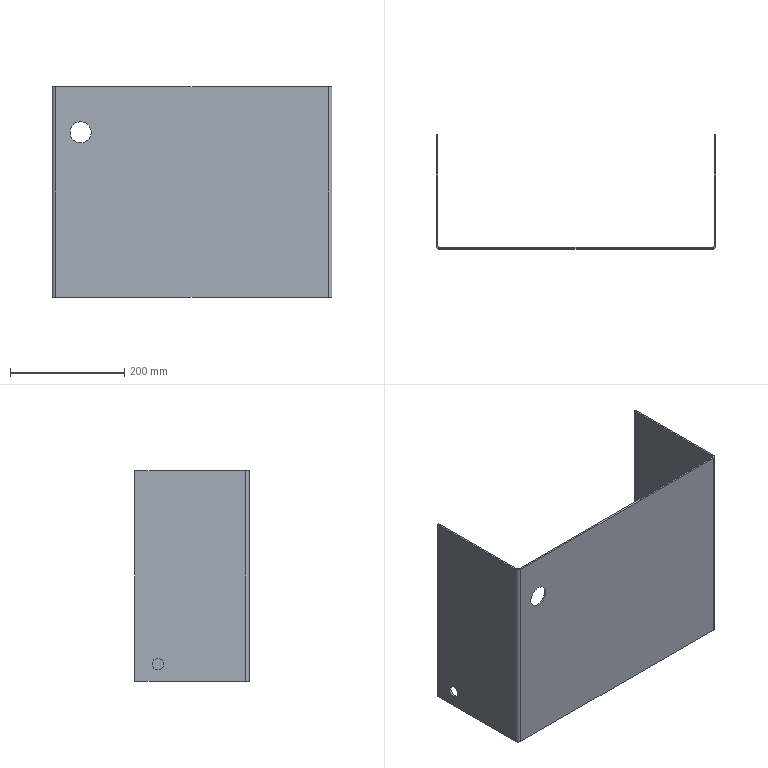Part | SolidWorks | features Cut 3, FlatPattern 1, SMBaseFlange 1, SheetMetal 1 | 1 solid | 30 faces | box 490 x 200 x 369 mm | volume 969574 mm3 | plane 18 | cylinder 12 | commonest cylinder face diameters 11 x4 6 x2 12 x2 20 x2 37 x2
STEP:
#1=CARTESIAN_POINT('',(487.,40.,184.5));
#2=VERTEX_POINT('',#1);
#3=CARTESIAN_POINT('',(487.,40.,195.5));
#4=VERTEX_POINT('',#3);
#5=CARTESIAN_POINT('',(487.,40.,190.));
#6=DIRECTION('',(-1.,0.,0.));
#7=DIRECTION('',(0.,0.,1.));
#8=AXIS2_PLACEMENT_3D('',#5,#6,#7);
#9=CIRCLE('',#8,5.5);
#10=EDGE_CURVE('',#2,#4,#9,.T.);
#11=ORIENTED_EDGE('',*,*,#10,.T.);
#12=CARTESIAN_POINT('',(490.,40.,195.5));
#13=VERTEX_POINT('',#12);
#14=CARTESIAN_POINT('',(480.,40.,195.5));
#15=DIRECTION('',(1.,0.,0.));
#16=VECTOR('',#15,1000.);
#17=LINE('',#14,#16);
#18=EDGE_CURVE('',#4,#13,#17,.T.);
#19=ORIENTED_EDGE('',*,*,#18,.T.);
#20=CARTESIAN_POINT('',(490.,40.,184.5));
#21=VERTEX_POINT('',#20);
#22=CARTESIAN_POINT('',(490.,40.,190.));
#23=DIRECTION('',(1.,0.,0.));
#24=DIRECTION('',(0.,0.,-1.));
#25=AXIS2_PLACEMENT_3D('',#22,#23,#24);
#26=CIRCLE('',#25,5.5);
#27=EDGE_CURVE('',#13,#21,#26,.T.);
#28=ORIENTED_EDGE('',*,*,#27,.T.);
#29=CARTESIAN_POINT('',(480.,40.,184.5));
#30=DIRECTION('',(1.,0.,0.));
#31=VECTOR('',#30,1000.);
#32=LINE('',#29,#31);
#33=EDGE_CURVE('',#2,#21,#32,.T.);
#34=ORIENTED_EDGE('',*,*,#33,.F.);
#35=EDGE_LOOP('',(#11,#19,#28,#34));
#36=FACE_OUTER_BOUND('',#35,.T.);
#37=CARTESIAN_POINT('',(480.,40.,190.));
#38=DIRECTION('',(1.,0.,0.));
#39=DIRECTION('',(0.,0.,-1.));
#40=AXIS2_PLACEMENT_3D('',#37,#38,#39);
#41=CYLINDRICAL_SURFACE('',#40,5.5);
#42=ADVANCED_FACE('',(#36),#41,.F.);
#43=CARTESIAN_POINT('',(487.,40.,34.5));
#44=VERTEX_POINT('',#43);
#45=CARTESIAN_POINT('',(487.,40.,45.5));
#46=VERTEX_POINT('',#45);
#47=CARTESIAN_POINT('',(487.,40.,40.));
#48=DIRECTION('',(-1.,0.,0.));
#49=DIRECTION('',(0.,0.,1.));
#50=AXIS2_PLACEMENT_3D('',#47,#48,#49);
#51=CIRCLE('',#50,5.5);
#52=EDGE_CURVE('',#44,#46,#51,.T.);
#53=ORIENTED_EDGE('',*,*,#52,.T.);
#54=CARTESIAN_POINT('',(490.,40.,45.5));
#55=VERTEX_POINT('',#54);
#56=CARTESIAN_POINT('',(480.,40.,45.5));
#57=DIRECTION('',(1.,0.,0.));
#58=VECTOR('',#57,1000.);
#59=LINE('',#56,#58);
#60=EDGE_CURVE('',#46,#55,#59,.T.);
#61=ORIENTED_EDGE('',*,*,#60,.T.);
#62=CARTESIAN_POINT('',(490.,40.,34.5));
#63=VERTEX_POINT('',#62);
#64=CARTESIAN_POINT('',(490.,40.,40.));
#65=DIRECTION('',(1.,0.,0.));
#66=DIRECTION('',(0.,0.,-1.));
#67=AXIS2_PLACEMENT_3D('',#64,#65,#66);
#68=CIRCLE('',#67,5.5);
#69=EDGE_CURVE('',#55,#63,#68,.T.);
#70=ORIENTED_EDGE('',*,*,#69,.T.);
#71=CARTESIAN_POINT('',(480.,40.,34.5));
#72=DIRECTION('',(1.,0.,0.));
#73=VECTOR('',#72,1000.);
#74=LINE('',#71,#73);
#75=EDGE_CURVE('',#44,#63,#74,.T.);
#76=ORIENTED_EDGE('',*,*,#75,.F.);
#77=EDGE_LOOP('',(#53,#61,#70,#76));
#78=FACE_OUTER_BOUND('',#77,.T.);
#79=CARTESIAN_POINT('',(480.,40.,40.));
#80=DIRECTION('',(1.,0.,0.));
#81=DIRECTION('',(0.,0.,-1.));
#82=AXIS2_PLACEMENT_3D('',#79,#80,#81);
#83=CYLINDRICAL_SURFACE('',#82,5.5);
#84=ADVANCED_FACE('',(#78),#83,.F.);
#85=CARTESIAN_POINT('',(50.,3.,270.5));
#86=VERTEX_POINT('',#85);
#87=CARTESIAN_POINT('',(50.,3.,307.5));
#88=VERTEX_POINT('',#87);
#89=CARTESIAN_POINT('',(50.,3.,289.));
#90=DIRECTION('',(0.,1.,0.));
#91=DIRECTION('',(0.,0.,1.));
#92=AXIS2_PLACEMENT_3D('',#89,#90,#91);
#93=CIRCLE('',#92,18.5);
#94=EDGE_CURVE('',#86,#88,#93,.T.);
#95=ORIENTED_EDGE('',*,*,#94,.T.);
#96=CARTESIAN_POINT('',(50.,0.,307.5));
#97=VERTEX_POINT('',#96);
#98=CARTESIAN_POINT('',(50.,10.,307.5));
#99=DIRECTION('',(0.,-1.,0.));
#100=VECTOR('',#99,1000.);
#101=LINE('',#98,#100);
#102=EDGE_CURVE('',#88,#97,#101,.T.);
#103=ORIENTED_EDGE('',*,*,#102,.T.);
#104=CARTESIAN_POINT('',(50.,0.,270.5));
#105=VERTEX_POINT('',#104);
#106=CARTESIAN_POINT('',(50.,0.,289.));
#107=DIRECTION('',(0.,-1.,0.));
#108=DIRECTION('',(0.,0.,-1.));
#109=AXIS2_PLACEMENT_3D('',#106,#107,#108);
#110=CIRCLE('',#109,18.5);
#111=EDGE_CURVE('',#97,#105,#110,.T.);
#112=ORIENTED_EDGE('',*,*,#111,.T.);
#113=CARTESIAN_POINT('',(50.,10.,270.5));
#114=DIRECTION('',(0.,-1.,0.));
#115=VECTOR('',#114,1000.);
#116=LINE('',#113,#115);
#117=EDGE_CURVE('',#86,#105,#116,.T.);
#118=ORIENTED_EDGE('',*,*,#117,.F.);
#119=EDGE_LOOP('',(#95,#103,#112,#118));
#120=FACE_OUTER_BOUND('',#119,.T.);
#121=CARTESIAN_POINT('',(50.,10.,289.));
#122=DIRECTION('',(0.,-1.,0.));
#123=DIRECTION('',(0.,0.,-1.));
#124=AXIS2_PLACEMENT_3D('',#121,#122,#123);
#125=CYLINDRICAL_SURFACE('',#124,18.5);
#126=ADVANCED_FACE('',(#120),#125,.F.);
#127=CARTESIAN_POINT('',(3.,160.,40.));
#128=VERTEX_POINT('',#127);
#129=CARTESIAN_POINT('',(3.,160.,20.));
#130=VERTEX_POINT('',#129);
#131=CARTESIAN_POINT('',(3.,160.,30.));
#132=DIRECTION('',(1.,0.,0.));
#133=DIRECTION('',(0.,0.,-1.));
#134=AXIS2_PLACEMENT_3D('',#131,#132,#133);
#135=CIRCLE('',#134,10.);
#136=EDGE_CURVE('',#128,#130,#135,.T.);
#137=ORIENTED_EDGE('',*,*,#136,.T.);
#138=CARTESIAN_POINT('',(0.,160.,20.));
#139=VERTEX_POINT('',#138);
#140=CARTESIAN_POINT('',(10.,160.,20.));
#141=DIRECTION('',(-1.,0.,0.));
#142=VECTOR('',#141,1000.);
#143=LINE('',#140,#142);
#144=EDGE_CURVE('',#130,#139,#143,.T.);
#145=ORIENTED_EDGE('',*,*,#144,.T.);
#146=CARTESIAN_POINT('',(0.,160.,40.));
#147=VERTEX_POINT('',#146);
#148=CARTESIAN_POINT('',(0.,160.,30.));
#149=DIRECTION('',(-1.,0.,0.));
#150=DIRECTION('',(0.,0.,1.));
#151=AXIS2_PLACEMENT_3D('',#148,#149,#150);
#152=CIRCLE('',#151,10.);
#153=EDGE_CURVE('',#139,#147,#152,.T.);
#154=ORIENTED_EDGE('',*,*,#153,.T.);
#155=CARTESIAN_POINT('',(10.,160.,40.));
#156=DIRECTION('',(-1.,0.,0.));
#157=VECTOR('',#156,1000.);
#158=LINE('',#155,#157);
#159=EDGE_CURVE('',#128,#147,#158,.T.);
#160=ORIENTED_EDGE('',*,*,#159,.F.);
#161=EDGE_LOOP('',(#137,#145,#154,#160));
#162=FACE_OUTER_BOUND('',#161,.T.);
#163=CARTESIAN_POINT('',(10.,160.,30.));
#164=DIRECTION('',(-1.,0.,0.));
#165=DIRECTION('',(0.,0.,1.));
#166=AXIS2_PLACEMENT_3D('',#163,#164,#165);
#167=CYLINDRICAL_SURFACE('',#166,10.);
#168=ADVANCED_FACE('',(#162),#167,.F.);
#169=CARTESIAN_POINT('',(0.,6.,369.));
#170=VERTEX_POINT('',#169);
#171=CARTESIAN_POINT('',(3.,6.,369.));
#172=VERTEX_POINT('',#171);
#173=CARTESIAN_POINT('',(0.,6.,369.));
#174=DIRECTION('',(1.,0.,0.));
#175=VECTOR('',#174,1000.);
#176=LINE('',#173,#175);
#177=EDGE_CURVE('',#170,#172,#176,.T.);
#178=ORIENTED_EDGE('',*,*,#177,.F.);
#179=CARTESIAN_POINT('',(6.,0.,369.));
#180=VERTEX_POINT('',#179);
#181=CARTESIAN_POINT('',(6.,6.,369.));
#182=DIRECTION('',(0.,0.,1.));
#183=DIRECTION('',(-1.,0.,0.));
#184=AXIS2_PLACEMENT_3D('',#181,#182,#183);
#185=CIRCLE('',#184,6.);
#186=EDGE_CURVE('',#170,#180,#185,.T.);
#187=ORIENTED_EDGE('',*,*,#186,.T.);
#188=CARTESIAN_POINT('',(6.,3.,369.));
#189=VERTEX_POINT('',#188);
#190=CARTESIAN_POINT('',(6.,3.,369.));
#191=DIRECTION('',(0.,-1.,0.));
#192=VECTOR('',#191,1000.);
#193=LINE('',#190,#192);
#194=EDGE_CURVE('',#189,#180,#193,.T.);
#195=ORIENTED_EDGE('',*,*,#194,.F.);
#196=CARTESIAN_POINT('',(6.,6.,369.));
#197=DIRECTION('',(0.,0.,1.));
#198=DIRECTION('',(1.,0.,0.));
#199=AXIS2_PLACEMENT_3D('',#196,#197,#198);
#200=CIRCLE('',#199,3.);
#201=EDGE_CURVE('',#172,#189,#200,.T.);
#202=ORIENTED_EDGE('',*,*,#201,.F.);
#203=EDGE_LOOP('',(#178,#187,#195,#202));
#204=FACE_OUTER_BOUND('',#203,.T.);
#205=CARTESIAN_POINT('',(0.,6.,369.));
#206=DIRECTION('',(0.,0.,1.));
#207=DIRECTION('',(1.,0.,0.));
#208=AXIS2_PLACEMENT_3D('',#205,#206,#207);
#209=PLANE('',#208);
#210=ADVANCED_FACE('',(#204),#209,.T.);
#211=CARTESIAN_POINT('',(0.,200.,369.));
#212=VERTEX_POINT('',#211);
#213=CARTESIAN_POINT('',(0.,0.,369.));
#214=DIRECTION('',(0.,-1.,0.));
#215=VECTOR('',#214,1000.);
#216=LINE('',#213,#215);
#217=EDGE_CURVE('',#212,#170,#216,.T.);
#218=ORIENTED_EDGE('',*,*,#217,.T.);
#219=ORIENTED_EDGE('',*,*,#177,.T.);
#220=CARTESIAN_POINT('',(3.,200.,369.));
#221=VERTEX_POINT('',#220);
#222=CARTESIAN_POINT('',(3.,0.,369.));
#223=DIRECTION('',(0.,-1.,0.));
#224=VECTOR('',#223,1000.);
#225=LINE('',#222,#224);
#226=EDGE_CURVE('',#221,#172,#225,.T.);
#227=ORIENTED_EDGE('',*,*,#226,.F.);
#228=CARTESIAN_POINT('',(0.,200.,369.));
#229=DIRECTION('',(1.,0.,0.));
#230=VECTOR('',#229,1000.);
#231=LINE('',#228,#230);
#232=EDGE_CURVE('',#212,#221,#231,.T.);
#233=ORIENTED_EDGE('',*,*,#232,.F.);
#234=EDGE_LOOP('',(#218,#219,#227,#233));
#235=FACE_OUTER_BOUND('',#234,.T.);
#236=CARTESIAN_POINT('',(6.,3.,369.));
#237=DIRECTION('',(0.,0.,1.));
#238=DIRECTION('',(1.,0.,0.));
#239=AXIS2_PLACEMENT_3D('',#236,#237,#238);
#240=PLANE('',#239);
#241=ADVANCED_FACE('',(#235),#240,.T.);
#242=CARTESIAN_POINT('',(6.,0.,0.));
#243=VERTEX_POINT('',#242);
#244=CARTESIAN_POINT('',(6.,3.,0.));
#245=VERTEX_POINT('',#244);
#246=CARTESIAN_POINT('',(6.,0.,0.));
#247=DIRECTION('',(0.,1.,0.));
#248=VECTOR('',#247,1000.);
#249=LINE('',#246,#248);
#250=EDGE_CURVE('',#243,#245,#249,.T.);
#251=ORIENTED_EDGE('',*,*,#250,.F.);
#252=CARTESIAN_POINT('',(0.,6.,0.));
#253=VERTEX_POINT('',#252);
#254=CARTESIAN_POINT('',(6.,6.,0.));
#255=DIRECTION('',(0.,0.,1.));
#256=DIRECTION('',(-1.,0.,0.));
#257=AXIS2_PLACEMENT_3D('',#254,#255,#256);
#258=CIRCLE('',#257,6.);
#259=EDGE_CURVE('',#253,#243,#258,.T.);
#260=ORIENTED_EDGE('',*,*,#259,.F.);
#261=CARTESIAN_POINT('',(3.,6.,0.));
#262=VERTEX_POINT('',#261);
#263=CARTESIAN_POINT('',(3.,6.,0.));
#264=DIRECTION('',(-1.,0.,0.));
#265=VECTOR('',#264,1000.);
#266=LINE('',#263,#265);
#267=EDGE_CURVE('',#262,#253,#266,.T.);
#268=ORIENTED_EDGE('',*,*,#267,.F.);
#269=CARTESIAN_POINT('',(6.,6.,0.));
#270=DIRECTION('',(0.,0.,1.));
#271=DIRECTION('',(1.,0.,0.));
#272=AXIS2_PLACEMENT_3D('',#269,#270,#271);
#273=CIRCLE('',#272,3.);
#274=EDGE_CURVE('',#262,#245,#273,.T.);
#275=ORIENTED_EDGE('',*,*,#274,.T.);
#276=EDGE_LOOP('',(#251,#260,#268,#275));
#277=FACE_OUTER_BOUND('',#276,.T.);
#278=CARTESIAN_POINT('',(6.,0.,0.));
#279=DIRECTION('',(0.,0.,-1.));
#280=DIRECTION('',(-1.,0.,0.));
#281=AXIS2_PLACEMENT_3D('',#278,#279,#280);
#282=PLANE('',#281);
#283=ADVANCED_FACE('',(#277),#282,.T.);
#284=CARTESIAN_POINT('',(484.,0.,0.));
#285=VERTEX_POINT('',#284);
#286=CARTESIAN_POINT('',(0.,0.,0.));
#287=DIRECTION('',(1.,0.,0.));
#288=VECTOR('',#287,1000.);
#289=LINE('',#286,#288);
#290=EDGE_CURVE('',#243,#285,#289,.T.);
#291=ORIENTED_EDGE('',*,*,#290,.F.);
#292=ORIENTED_EDGE('',*,*,#250,.T.);
#293=CARTESIAN_POINT('',(484.,3.,0.));
#294=VERTEX_POINT('',#293);
#295=CARTESIAN_POINT('',(0.,3.,0.));
#296=DIRECTION('',(1.,0.,0.));
#297=VECTOR('',#296,1000.);
#298=LINE('',#295,#297);
#299=EDGE_CURVE('',#245,#294,#298,.T.);
#300=ORIENTED_EDGE('',*,*,#299,.T.);
#301=CARTESIAN_POINT('',(484.,3.,0.));
#302=DIRECTION('',(0.,-1.,0.));
#303=VECTOR('',#302,1000.);
#304=LINE('',#301,#303);
#305=EDGE_CURVE('',#294,#285,#304,.T.);
#306=ORIENTED_EDGE('',*,*,#305,.T.);
#307=EDGE_LOOP('',(#291,#292,#300,#306));
#308=FACE_OUTER_BOUND('',#307,.T.);
#309=CARTESIAN_POINT('',(3.,6.,0.));
#310=DIRECTION('',(0.,0.,-1.));
#311=DIRECTION('',(-1.,0.,0.));
#312=AXIS2_PLACEMENT_3D('',#309,#310,#311);
#313=PLANE('',#312);
#314=ADVANCED_FACE('',(#308),#313,.T.);
#315=CARTESIAN_POINT('',(484.,0.,369.));
#316=VERTEX_POINT('',#315);
#317=CARTESIAN_POINT('',(484.,3.,369.));
#318=VERTEX_POINT('',#317);
#319=CARTESIAN_POINT('',(484.,0.,369.));
#320=DIRECTION('',(0.,1.,0.));
#321=VECTOR('',#320,1000.);
#322=LINE('',#319,#321);
#323=EDGE_CURVE('',#316,#318,#322,.T.);
#324=ORIENTED_EDGE('',*,*,#323,.F.);
#325=CARTESIAN_POINT('',(490.,6.,369.));
#326=VERTEX_POINT('',#325);
#327=CARTESIAN_POINT('',(484.,6.,369.));
#328=DIRECTION('',(0.,0.,1.));
#329=DIRECTION('',(-1.,0.,0.));
#330=AXIS2_PLACEMENT_3D('',#327,#328,#329);
#331=CIRCLE('',#330,6.);
#332=EDGE_CURVE('',#316,#326,#331,.T.);
#333=ORIENTED_EDGE('',*,*,#332,.T.);
#334=CARTESIAN_POINT('',(487.,6.,369.));
#335=VERTEX_POINT('',#334);
#336=CARTESIAN_POINT('',(487.,6.,369.));
#337=DIRECTION('',(1.,0.,0.));
#338=VECTOR('',#337,1000.);
#339=LINE('',#336,#338);
#340=EDGE_CURVE('',#335,#326,#339,.T.);
#341=ORIENTED_EDGE('',*,*,#340,.F.);
#342=CARTESIAN_POINT('',(484.,6.,369.));
#343=DIRECTION('',(0.,0.,1.));
#344=DIRECTION('',(1.,0.,0.));
#345=AXIS2_PLACEMENT_3D('',#342,#343,#344);
#346=CIRCLE('',#345,3.);
#347=EDGE_CURVE('',#318,#335,#346,.T.);
#348=ORIENTED_EDGE('',*,*,#347,.F.);
#349=EDGE_LOOP('',(#324,#333,#341,#348));
#350=FACE_OUTER_BOUND('',#349,.T.);
#351=CARTESIAN_POINT('',(484.,0.,369.));
#352=DIRECTION('',(0.,0.,1.));
#353=DIRECTION('',(1.,0.,0.));
#354=AXIS2_PLACEMENT_3D('',#351,#352,#353);
#355=PLANE('',#354);
#356=ADVANCED_FACE('',(#350),#355,.T.);
#357=CARTESIAN_POINT('',(0.,0.,369.));
#358=DIRECTION('',(1.,0.,0.));
#359=VECTOR('',#358,1000.);
#360=LINE('',#357,#359);
#361=EDGE_CURVE('',#180,#316,#360,.T.);
#362=ORIENTED_EDGE('',*,*,#361,.T.);
#363=ORIENTED_EDGE('',*,*,#323,.T.);
#364=CARTESIAN_POINT('',(0.,3.,369.));
#365=DIRECTION('',(1.,0.,0.));
#366=VECTOR('',#365,1000.);
#367=LINE('',#364,#366);
#368=EDGE_CURVE('',#189,#318,#367,.T.);
#369=ORIENTED_EDGE('',*,*,#368,.F.);
#370=ORIENTED_EDGE('',*,*,#194,.T.);
#371=EDGE_LOOP('',(#362,#363,#369,#370));
#372=FACE_OUTER_BOUND('',#371,.T.);
#373=CARTESIAN_POINT('',(487.,6.,369.));
#374=DIRECTION('',(0.,0.,1.));
#375=DIRECTION('',(1.,0.,0.));
#376=AXIS2_PLACEMENT_3D('',#373,#374,#375);
#377=PLANE('',#376);
#378=ADVANCED_FACE('',(#372),#377,.T.);
#379=CARTESIAN_POINT('',(490.,6.,0.));
#380=VERTEX_POINT('',#379);
#381=CARTESIAN_POINT('',(487.,6.,0.));
#382=VERTEX_POINT('',#381);
#383=CARTESIAN_POINT('',(490.,6.,0.));
#384=DIRECTION('',(-1.,0.,0.));
#385=VECTOR('',#384,1000.);
#386=LINE('',#383,#385);
#387=EDGE_CURVE('',#380,#382,#386,.T.);
#388=ORIENTED_EDGE('',*,*,#387,.F.);
#389=CARTESIAN_POINT('',(484.,6.,0.));
#390=DIRECTION('',(0.,0.,1.));
#391=DIRECTION('',(-1.,0.,0.));
#392=AXIS2_PLACEMENT_3D('',#389,#390,#391);
#393=CIRCLE('',#392,6.);
#394=EDGE_CURVE('',#285,#380,#393,.T.);
#395=ORIENTED_EDGE('',*,*,#394,.F.);
#396=ORIENTED_EDGE('',*,*,#305,.F.);
#397=CARTESIAN_POINT('',(484.,6.,0.));
#398=DIRECTION('',(0.,0.,1.));
#399=DIRECTION('',(1.,0.,0.));
#400=AXIS2_PLACEMENT_3D('',#397,#398,#399);
#401=CIRCLE('',#400,3.);
#402=EDGE_CURVE('',#294,#382,#401,.T.);
#403=ORIENTED_EDGE('',*,*,#402,.T.);
#404=EDGE_LOOP('',(#388,#395,#396,#403));
#405=FACE_OUTER_BOUND('',#404,.T.);
#406=CARTESIAN_POINT('',(490.,6.,0.));
#407=DIRECTION('',(0.,0.,-1.));
#408=DIRECTION('',(-1.,0.,0.));
#409=AXIS2_PLACEMENT_3D('',#406,#407,#408);
#410=PLANE('',#409);
#411=ADVANCED_FACE('',(#405),#410,.T.);
#412=CARTESIAN_POINT('',(490.,200.,0.));
#413=VERTEX_POINT('',#412);
#414=CARTESIAN_POINT('',(490.,0.,0.));
#415=DIRECTION('',(0.,1.,0.));
#416=VECTOR('',#415,1000.);
#417=LINE('',#414,#416);
#418=EDGE_CURVE('',#380,#413,#417,.T.);
#419=ORIENTED_EDGE('',*,*,#418,.F.);
#420=ORIENTED_EDGE('',*,*,#387,.T.);
#421=CARTESIAN_POINT('',(487.,200.,0.));
#422=VERTEX_POINT('',#421);
#423=CARTESIAN_POINT('',(487.,0.,0.));
#424=DIRECTION('',(0.,1.,0.));
#425=VECTOR('',#424,1000.);
#426=LINE('',#423,#425);
#427=EDGE_CURVE('',#382,#422,#426,.T.);
#428=ORIENTED_EDGE('',*,*,#427,.T.);
#429=CARTESIAN_POINT('',(487.,200.,0.));
#430=DIRECTION('',(1.,0.,0.));
#431=VECTOR('',#430,1000.);
#432=LINE('',#429,#431);
#433=EDGE_CURVE('',#422,#413,#432,.T.);
#434=ORIENTED_EDGE('',*,*,#433,.T.);
#435=EDGE_LOOP('',(#419,#420,#428,#434));
#436=FACE_OUTER_BOUND('',#435,.T.);
#437=CARTESIAN_POINT('',(484.,3.,0.));
#438=DIRECTION('',(0.,0.,-1.));
#439=DIRECTION('',(-1.,0.,0.));
#440=AXIS2_PLACEMENT_3D('',#437,#438,#439);
#441=PLANE('',#440);
#442=ADVANCED_FACE('',(#436),#441,.T.);
#443=CARTESIAN_POINT('',(490.,40.,190.));
#444=DIRECTION('',(1.,0.,0.));
#445=DIRECTION('',(0.,0.,-1.));
#446=AXIS2_PLACEMENT_3D('',#443,#444,#445);
#447=CIRCLE('',#446,5.5);
#448=EDGE_CURVE('',#21,#13,#447,.T.);
#449=ORIENTED_EDGE('',*,*,#448,.F.);
#450=ORIENTED_EDGE('',*,*,#27,.F.);
#451=EDGE_LOOP('',(#449,#450));
#452=FACE_BOUND('',#451,.T.);
#453=CARTESIAN_POINT('',(490.,40.,40.));
#454=DIRECTION('',(1.,0.,0.));
#455=DIRECTION('',(0.,0.,-1.));
#456=AXIS2_PLACEMENT_3D('',#453,#454,#455);
#457=CIRCLE('',#456,5.5);
#458=EDGE_CURVE('',#63,#55,#457,.T.);
#459=ORIENTED_EDGE('',*,*,#458,.F.);
#460=ORIENTED_EDGE('',*,*,#69,.F.);
#461=EDGE_LOOP('',(#459,#460));
#462=FACE_BOUND('',#461,.T.);
#463=ORIENTED_EDGE('',*,*,#418,.T.);
#464=CARTESIAN_POINT('',(490.,200.,369.));
#465=VERTEX_POINT('',#464);
#466=CARTESIAN_POINT('',(490.,200.,369.));
#467=DIRECTION('',(0.,0.,-1.));
#468=VECTOR('',#467,1000.);
#469=LINE('',#466,#468);
#470=EDGE_CURVE('',#465,#413,#469,.T.);
#471=ORIENTED_EDGE('',*,*,#470,.F.);
#472=CARTESIAN_POINT('',(490.,0.,369.));
#473=DIRECTION('',(0.,1.,0.));
#474=VECTOR('',#473,1000.);
#475=LINE('',#472,#474);
#476=EDGE_CURVE('',#326,#465,#475,.T.);
#477=ORIENTED_EDGE('',*,*,#476,.F.);
#478=CARTESIAN_POINT('',(490.,6.,369.));
#479=DIRECTION('',(0.,0.,-1.));
#480=VECTOR('',#479,1000.);
#481=LINE('',#478,#480);
#482=EDGE_CURVE('',#326,#380,#481,.T.);
#483=ORIENTED_EDGE('',*,*,#482,.T.);
#484=EDGE_LOOP('',(#463,#471,#477,#483));
#485=FACE_OUTER_BOUND('',#484,.T.);
#486=CARTESIAN_POINT('',(490.,0.,369.));
#487=DIRECTION('',(-1.,0.,0.));
#488=DIRECTION('',(0.,0.,1.));
#489=AXIS2_PLACEMENT_3D('',#486,#487,#488);
#490=PLANE('',#489);
#491=ADVANCED_FACE('',(#452,#462,#485),#490,.F.);
#492=ORIENTED_EDGE('',*,*,#433,.F.);
#493=CARTESIAN_POINT('',(487.,200.,369.));
#494=VERTEX_POINT('',#493);
#495=CARTESIAN_POINT('',(487.,200.,369.));
#496=DIRECTION('',(0.,0.,-1.));
#497=VECTOR('',#496,1000.);
#498=LINE('',#495,#497);
#499=EDGE_CURVE('',#494,#422,#498,.T.);
#500=ORIENTED_EDGE('',*,*,#499,.F.);
#501=CARTESIAN_POINT('',(487.,200.,369.));
#502=DIRECTION('',(1.,0.,0.));
#503=VECTOR('',#502,1000.);
#504=LINE('',#501,#503);
#505=EDGE_CURVE('',#494,#465,#504,.T.);
#506=ORIENTED_EDGE('',*,*,#505,.T.);
#507=ORIENTED_EDGE('',*,*,#470,.T.);
#508=EDGE_LOOP('',(#492,#500,#506,#507));
#509=FACE_OUTER_BOUND('',#508,.T.);
#510=CARTESIAN_POINT('',(487.,200.,369.));
#511=DIRECTION('',(0.,1.,0.));
#512=DIRECTION('',(0.,0.,1.));
#513=AXIS2_PLACEMENT_3D('',#510,#511,#512);
#514=PLANE('',#513);
#515=ADVANCED_FACE('',(#509),#514,.T.);
#516=ORIENTED_EDGE('',*,*,#10,.F.);
#517=CARTESIAN_POINT('',(487.,40.,190.));
#518=DIRECTION('',(-1.,0.,0.));
#519=DIRECTION('',(0.,0.,1.));
#520=AXIS2_PLACEMENT_3D('',#517,#518,#519);
#521=CIRCLE('',#520,5.5);
#522=EDGE_CURVE('',#4,#2,#521,.T.);
#523=ORIENTED_EDGE('',*,*,#522,.F.);
#524=EDGE_LOOP('',(#516,#523));
#525=FACE_BOUND('',#524,.T.);
#526=ORIENTED_EDGE('',*,*,#52,.F.);
#527=CARTESIAN_POINT('',(487.,40.,40.));
#528=DIRECTION('',(-1.,0.,0.));
#529=DIRECTION('',(0.,0.,1.));
#530=AXIS2_PLACEMENT_3D('',#527,#528,#529);
#531=CIRCLE('',#530,5.5);
#532=EDGE_CURVE('',#46,#44,#531,.T.);
#533=ORIENTED_EDGE('',*,*,#532,.F.);
#534=EDGE_LOOP('',(#526,#533));
#535=FACE_BOUND('',#534,.T.);
#536=ORIENTED_EDGE('',*,*,#427,.F.);
#537=CARTESIAN_POINT('',(487.,6.,369.));
#538=DIRECTION('',(0.,0.,-1.));
#539=VECTOR('',#538,1000.);
#540=LINE('',#537,#539);
#541=EDGE_CURVE('',#335,#382,#540,.T.);
#542=ORIENTED_EDGE('',*,*,#541,.F.);
#543=CARTESIAN_POINT('',(487.,0.,369.));
#544=DIRECTION('',(0.,1.,0.));
#545=VECTOR('',#544,1000.);
#546=LINE('',#543,#545);
#547=EDGE_CURVE('',#335,#494,#546,.T.);
#548=ORIENTED_EDGE('',*,*,#547,.T.);
#549=ORIENTED_EDGE('',*,*,#499,.T.);
#550=EDGE_LOOP('',(#536,#542,#548,#549));
#551=FACE_OUTER_BOUND('',#550,.T.);
#552=CARTESIAN_POINT('',(487.,0.,369.));
#553=DIRECTION('',(-1.,0.,0.));
#554=DIRECTION('',(0.,0.,1.));
#555=AXIS2_PLACEMENT_3D('',#552,#553,#554);
#556=PLANE('',#555);
#557=ADVANCED_FACE('',(#525,#535,#551),#556,.T.);
#558=ORIENTED_EDGE('',*,*,#402,.F.);
#559=CARTESIAN_POINT('',(484.,3.,369.));
#560=DIRECTION('',(0.,0.,-1.));
#561=VECTOR('',#560,1000.);
#562=LINE('',#559,#561);
#563=EDGE_CURVE('',#318,#294,#562,.T.);
#564=ORIENTED_EDGE('',*,*,#563,.F.);
#565=ORIENTED_EDGE('',*,*,#347,.T.);
#566=ORIENTED_EDGE('',*,*,#541,.T.);
#567=EDGE_LOOP('',(#558,#564,#565,#566));
#568=FACE_OUTER_BOUND('',#567,.T.);
#569=CARTESIAN_POINT('',(484.,6.,369.));
#570=DIRECTION('',(0.,0.,-1.));
#571=DIRECTION('',(-1.,0.,0.));
#572=AXIS2_PLACEMENT_3D('',#569,#570,#571);
#573=CYLINDRICAL_SURFACE('',#572,3.);
#574=ADVANCED_FACE('',(#568),#573,.F.);
#575=ORIENTED_EDGE('',*,*,#94,.F.);
#576=CARTESIAN_POINT('',(50.,3.,289.));
#577=DIRECTION('',(0.,1.,0.));
#578=DIRECTION('',(0.,0.,1.));
#579=AXIS2_PLACEMENT_3D('',#576,#577,#578);
#580=CIRCLE('',#579,18.5);
#581=EDGE_CURVE('',#88,#86,#580,.T.);
#582=ORIENTED_EDGE('',*,*,#581,.F.);
#583=EDGE_LOOP('',(#575,#582));
#584=FACE_BOUND('',#583,.T.);
#585=ORIENTED_EDGE('',*,*,#299,.F.);
#586=CARTESIAN_POINT('',(6.,3.,369.));
#587=DIRECTION('',(0.,0.,-1.));
#588=VECTOR('',#587,1000.);
#589=LINE('',#586,#588);
#590=EDGE_CURVE('',#189,#245,#589,.T.);
#591=ORIENTED_EDGE('',*,*,#590,.F.);
#592=ORIENTED_EDGE('',*,*,#368,.T.);
#593=ORIENTED_EDGE('',*,*,#563,.T.);
#594=EDGE_LOOP('',(#585,#591,#592,#593));
#595=FACE_OUTER_BOUND('',#594,.T.);
#596=CARTESIAN_POINT('',(0.,3.,369.));
#597=DIRECTION('',(0.,1.,0.));
#598=DIRECTION('',(0.,0.,1.));
#599=AXIS2_PLACEMENT_3D('',#596,#597,#598);
#600=PLANE('',#599);
#601=ADVANCED_FACE('',(#584,#595),#600,.T.);
#602=ORIENTED_EDGE('',*,*,#274,.F.);
#603=CARTESIAN_POINT('',(3.,6.,369.));
#604=DIRECTION('',(0.,0.,-1.));
#605=VECTOR('',#604,1000.);
#606=LINE('',#603,#605);
#607=EDGE_CURVE('',#172,#262,#606,.T.);
#608=ORIENTED_EDGE('',*,*,#607,.F.);
#609=ORIENTED_EDGE('',*,*,#201,.T.);
#610=ORIENTED_EDGE('',*,*,#590,.T.);
#611=EDGE_LOOP('',(#602,#608,#609,#610));
#612=FACE_OUTER_BOUND('',#611,.T.);
#613=CARTESIAN_POINT('',(6.,6.,369.));
#614=DIRECTION('',(0.,0.,-1.));
#615=DIRECTION('',(-1.,0.,0.));
#616=AXIS2_PLACEMENT_3D('',#613,#614,#615);
#617=CYLINDRICAL_SURFACE('',#616,3.);
#618=ADVANCED_FACE('',(#612),#617,.F.);
#619=ORIENTED_EDGE('',*,*,#136,.F.);
#620=CARTESIAN_POINT('',(3.,160.,30.));
#621=DIRECTION('',(1.,0.,0.));
#622=DIRECTION('',(0.,0.,-1.));
#623=AXIS2_PLACEMENT_3D('',#620,#621,#622);
#624=CIRCLE('',#623,10.);
#625=EDGE_CURVE('',#130,#128,#624,.T.);
#626=ORIENTED_EDGE('',*,*,#625,.F.);
#627=EDGE_LOOP('',(#619,#626));
#628=FACE_BOUND('',#627,.T.);
#629=CARTESIAN_POINT('',(3.,200.,0.));
#630=VERTEX_POINT('',#629);
#631=CARTESIAN_POINT('',(3.,0.,0.));
#632=DIRECTION('',(0.,-1.,0.));
#633=VECTOR('',#632,1000.);
#634=LINE('',#631,#633);
#635=EDGE_CURVE('',#630,#262,#634,.T.);
#636=ORIENTED_EDGE('',*,*,#635,.F.);
#637=CARTESIAN_POINT('',(3.,200.,369.));
#638=DIRECTION('',(0.,0.,-1.));
#639=VECTOR('',#638,1000.);
#640=LINE('',#637,#639);
#641=EDGE_CURVE('',#221,#630,#640,.T.);
#642=ORIENTED_EDGE('',*,*,#641,.F.);
#643=ORIENTED_EDGE('',*,*,#226,.T.);
#644=ORIENTED_EDGE('',*,*,#607,.T.);
#645=EDGE_LOOP('',(#636,#642,#643,#644));
#646=FACE_OUTER_BOUND('',#645,.T.);
#647=CARTESIAN_POINT('',(3.,0.,369.));
#648=DIRECTION('',(1.,0.,0.));
#649=DIRECTION('',(0.,0.,-1.));
#650=AXIS2_PLACEMENT_3D('',#647,#648,#649);
#651=PLANE('',#650);
#652=ADVANCED_FACE('',(#628,#646),#651,.T.);
#653=CARTESIAN_POINT('',(0.,200.,0.));
#654=VERTEX_POINT('',#653);
#655=CARTESIAN_POINT('',(0.,200.,0.));
#656=DIRECTION('',(1.,0.,0.));
#657=VECTOR('',#656,1000.);
#658=LINE('',#655,#657);
#659=EDGE_CURVE('',#654,#630,#658,.T.);
#660=ORIENTED_EDGE('',*,*,#659,.F.);
#661=CARTESIAN_POINT('',(0.,200.,369.));
#662=DIRECTION('',(0.,0.,-1.));
#663=VECTOR('',#662,1000.);
#664=LINE('',#661,#663);
#665=EDGE_CURVE('',#212,#654,#664,.T.);
#666=ORIENTED_EDGE('',*,*,#665,.F.);
#667=ORIENTED_EDGE('',*,*,#232,.T.);
#668=ORIENTED_EDGE('',*,*,#641,.T.);
#669=EDGE_LOOP('',(#660,#666,#667,#668));
#670=FACE_OUTER_BOUND('',#669,.T.);
#671=CARTESIAN_POINT('',(0.,200.,369.));
#672=DIRECTION('',(0.,1.,0.));
#673=DIRECTION('',(0.,0.,1.));
#674=AXIS2_PLACEMENT_3D('',#671,#672,#673);
#675=PLANE('',#674);
#676=ADVANCED_FACE('',(#670),#675,.T.);
#677=CARTESIAN_POINT('',(0.,160.,30.));
#678=DIRECTION('',(-1.,0.,0.));
#679=DIRECTION('',(0.,0.,1.));
#680=AXIS2_PLACEMENT_3D('',#677,#678,#679);
#681=CIRCLE('',#680,10.);
#682=EDGE_CURVE('',#147,#139,#681,.T.);
#683=ORIENTED_EDGE('',*,*,#682,.F.);
#684=ORIENTED_EDGE('',*,*,#153,.F.);
#685=EDGE_LOOP('',(#683,#684));
#686=FACE_BOUND('',#685,.T.);
#687=CARTESIAN_POINT('',(0.,0.,0.));
#688=DIRECTION('',(0.,-1.,0.));
#689=VECTOR('',#688,1000.);
#690=LINE('',#687,#689);
#691=EDGE_CURVE('',#654,#253,#690,.T.);
#692=ORIENTED_EDGE('',*,*,#691,.T.);
#693=CARTESIAN_POINT('',(0.,6.,369.));
#694=DIRECTION('',(0.,0.,-1.));
#695=VECTOR('',#694,1000.);
#696=LINE('',#693,#695);
#697=EDGE_CURVE('',#170,#253,#696,.T.);
#698=ORIENTED_EDGE('',*,*,#697,.F.);
#699=ORIENTED_EDGE('',*,*,#217,.F.);
#700=ORIENTED_EDGE('',*,*,#665,.T.);
#701=EDGE_LOOP('',(#692,#698,#699,#700));
#702=FACE_OUTER_BOUND('',#701,.T.);
#703=CARTESIAN_POINT('',(0.,0.,369.));
#704=DIRECTION('',(1.,0.,0.));
#705=DIRECTION('',(0.,0.,-1.));
#706=AXIS2_PLACEMENT_3D('',#703,#704,#705);
#707=PLANE('',#706);
#708=ADVANCED_FACE('',(#686,#702),#707,.F.);
#709=ORIENTED_EDGE('',*,*,#259,.T.);
#710=CARTESIAN_POINT('',(6.,0.,369.));
#711=DIRECTION('',(0.,0.,-1.));
#712=VECTOR('',#711,1000.);
#713=LINE('',#710,#712);
#714=EDGE_CURVE('',#180,#243,#713,.T.);
#715=ORIENTED_EDGE('',*,*,#714,.F.);
#716=ORIENTED_EDGE('',*,*,#186,.F.);
#717=ORIENTED_EDGE('',*,*,#697,.T.);
#718=EDGE_LOOP('',(#709,#715,#716,#717));
#719=FACE_OUTER_BOUND('',#718,.T.);
#720=CARTESIAN_POINT('',(6.,6.,369.));
#721=DIRECTION('',(0.,0.,-1.));
#722=DIRECTION('',(-1.,0.,0.));
#723=AXIS2_PLACEMENT_3D('',#720,#721,#722);
#724=CYLINDRICAL_SURFACE('',#723,6.);
#725=ADVANCED_FACE('',(#719),#724,.T.);
#726=CARTESIAN_POINT('',(50.,0.,289.));
#727=DIRECTION('',(0.,-1.,0.));
#728=DIRECTION('',(0.,0.,-1.));
#729=AXIS2_PLACEMENT_3D('',#726,#727,#728);
#730=CIRCLE('',#729,18.5);
#731=EDGE_CURVE('',#105,#97,#730,.T.);
#732=ORIENTED_EDGE('',*,*,#731,.F.);
#733=ORIENTED_EDGE('',*,*,#111,.F.);
#734=EDGE_LOOP('',(#732,#733));
#735=FACE_BOUND('',#734,.T.);
#736=ORIENTED_EDGE('',*,*,#290,.T.);
#737=CARTESIAN_POINT('',(484.,0.,369.));
#738=DIRECTION('',(0.,0.,-1.));
#739=VECTOR('',#738,1000.);
#740=LINE('',#737,#739);
#741=EDGE_CURVE('',#316,#285,#740,.T.);
#742=ORIENTED_EDGE('',*,*,#741,.F.);
#743=ORIENTED_EDGE('',*,*,#361,.F.);
#744=ORIENTED_EDGE('',*,*,#714,.T.);
#745=EDGE_LOOP('',(#736,#742,#743,#744));
#746=FACE_OUTER_BOUND('',#745,.T.);
#747=CARTESIAN_POINT('',(0.,0.,369.));
#748=DIRECTION('',(0.,1.,0.));
#749=DIRECTION('',(0.,0.,1.));
#750=AXIS2_PLACEMENT_3D('',#747,#748,#749);
#751=PLANE('',#750);
#752=ADVANCED_FACE('',(#735,#746),#751,.F.);
#753=ORIENTED_EDGE('',*,*,#394,.T.);
#754=ORIENTED_EDGE('',*,*,#482,.F.);
#755=ORIENTED_EDGE('',*,*,#332,.F.);
#756=ORIENTED_EDGE('',*,*,#741,.T.);
#757=EDGE_LOOP('',(#753,#754,#755,#756));
#758=FACE_OUTER_BOUND('',#757,.T.);
#759=CARTESIAN_POINT('',(484.,6.,369.));
#760=DIRECTION('',(0.,0.,-1.));
#761=DIRECTION('',(-1.,0.,0.));
#762=AXIS2_PLACEMENT_3D('',#759,#760,#761);
#763=CYLINDRICAL_SURFACE('',#762,6.);
#764=ADVANCED_FACE('',(#758),#763,.T.);
#765=ORIENTED_EDGE('',*,*,#476,.T.);
#766=ORIENTED_EDGE('',*,*,#505,.F.);
#767=ORIENTED_EDGE('',*,*,#547,.F.);
#768=ORIENTED_EDGE('',*,*,#340,.T.);
#769=EDGE_LOOP('',(#765,#766,#767,#768));
#770=FACE_OUTER_BOUND('',#769,.T.);
#771=CARTESIAN_POINT('',(484.,6.,369.));
#772=DIRECTION('',(0.,0.,1.));
#773=DIRECTION('',(1.,0.,0.));
#774=AXIS2_PLACEMENT_3D('',#771,#772,#773);
#775=PLANE('',#774);
#776=ADVANCED_FACE('',(#770),#775,.T.);
#777=ORIENTED_EDGE('',*,*,#635,.T.);
#778=ORIENTED_EDGE('',*,*,#267,.T.);
#779=ORIENTED_EDGE('',*,*,#691,.F.);
#780=ORIENTED_EDGE('',*,*,#659,.T.);
#781=EDGE_LOOP('',(#777,#778,#779,#780));
#782=FACE_OUTER_BOUND('',#781,.T.);
#783=CARTESIAN_POINT('',(484.,6.,0.));
#784=DIRECTION('',(0.,0.,1.));
#785=DIRECTION('',(1.,0.,0.));
#786=AXIS2_PLACEMENT_3D('',#783,#784,#785);
#787=PLANE('',#786);
#788=ADVANCED_FACE('',(#782),#787,.F.);
#789=ORIENTED_EDGE('',*,*,#144,.F.);
#790=ORIENTED_EDGE('',*,*,#625,.T.);
#791=ORIENTED_EDGE('',*,*,#159,.T.);
#792=ORIENTED_EDGE('',*,*,#682,.T.);
#793=EDGE_LOOP('',(#789,#790,#791,#792));
#794=FACE_OUTER_BOUND('',#793,.T.);
#795=CARTESIAN_POINT('',(10.,160.,30.));
#796=DIRECTION('',(-1.,0.,0.));
#797=DIRECTION('',(0.,0.,1.));
#798=AXIS2_PLACEMENT_3D('',#795,#796,#797);
#799=CYLINDRICAL_SURFACE('',#798,10.);
#800=ADVANCED_FACE('',(#794),#799,.F.);
#801=ORIENTED_EDGE('',*,*,#102,.F.);
#802=ORIENTED_EDGE('',*,*,#581,.T.);
#803=ORIENTED_EDGE('',*,*,#117,.T.);
#804=ORIENTED_EDGE('',*,*,#731,.T.);
#805=EDGE_LOOP('',(#801,#802,#803,#804));
#806=FACE_OUTER_BOUND('',#805,.T.);
#807=CARTESIAN_POINT('',(50.,10.,289.));
#808=DIRECTION('',(0.,-1.,0.));
#809=DIRECTION('',(0.,0.,-1.));
#810=AXIS2_PLACEMENT_3D('',#807,#808,#809);
#811=CYLINDRICAL_SURFACE('',#810,18.5);
#812=ADVANCED_FACE('',(#806),#811,.F.);
#813=ORIENTED_EDGE('',*,*,#60,.F.);
#814=ORIENTED_EDGE('',*,*,#532,.T.);
#815=ORIENTED_EDGE('',*,*,#75,.T.);
#816=ORIENTED_EDGE('',*,*,#458,.T.);
#817=EDGE_LOOP('',(#813,#814,#815,#816));
#818=FACE_OUTER_BOUND('',#817,.T.);
#819=CARTESIAN_POINT('',(480.,40.,40.));
#820=DIRECTION('',(1.,0.,0.));
#821=DIRECTION('',(0.,0.,-1.));
#822=AXIS2_PLACEMENT_3D('',#819,#820,#821);
#823=CYLINDRICAL_SURFACE('',#822,5.5);
#824=ADVANCED_FACE('',(#818),#823,.F.);
#825=ORIENTED_EDGE('',*,*,#18,.F.);
#826=ORIENTED_EDGE('',*,*,#522,.T.);
#827=ORIENTED_EDGE('',*,*,#33,.T.);
#828=ORIENTED_EDGE('',*,*,#448,.T.);
#829=EDGE_LOOP('',(#825,#826,#827,#828));
#830=FACE_OUTER_BOUND('',#829,.T.);
#831=CARTESIAN_POINT('',(480.,40.,190.));
#832=DIRECTION('',(1.,0.,0.));
#833=DIRECTION('',(0.,0.,-1.));
#834=AXIS2_PLACEMENT_3D('',#831,#832,#833);
#835=CYLINDRICAL_SURFACE('',#834,5.5);
#836=ADVANCED_FACE('',(#830),#835,.F.);
#837=CLOSED_SHELL('',(#42,#84,#126,#168,#210,#241,#283,#314,#356,#378,#411,#442,#491,#515,#557,#574,#601,#618,#652,#676,#708,#725,#752,#764,#776,#788,#800,#812,#824,#836));
#838=MANIFOLD_SOLID_BREP('',#837);
#839=CARTESIAN_POINT('',(0.,0.,0.));
#840=DIRECTION('',(0.,0.,1.));
#841=DIRECTION('',(1.,0.,0.));
#842=AXIS2_PLACEMENT_3D('',#839,#840,#841);
#843=(LENGTH_UNIT()NAMED_UNIT(*)SI_UNIT(.MILLI.,.METRE.));
#844=UNCERTAINTY_MEASURE_WITH_UNIT(LENGTH_MEASURE(0.00001),#843,'','');
#845=(NAMED_UNIT(*)PLANE_ANGLE_UNIT()SI_UNIT($,.RADIAN.));
#846=(NAMED_UNIT(*)SI_UNIT($,.STERADIAN.)SOLID_ANGLE_UNIT());
#847=(GEOMETRIC_REPRESENTATION_CONTEXT(3)GLOBAL_UNCERTAINTY_ASSIGNED_CONTEXT((#844))GLOBAL_UNIT_ASSIGNED_CONTEXT((#843,#845,#846))REPRESENTATION_CONTEXT('',''));
#848=ADVANCED_BREP_SHAPE_REPRESENTATION('',(#838,#842),#847);